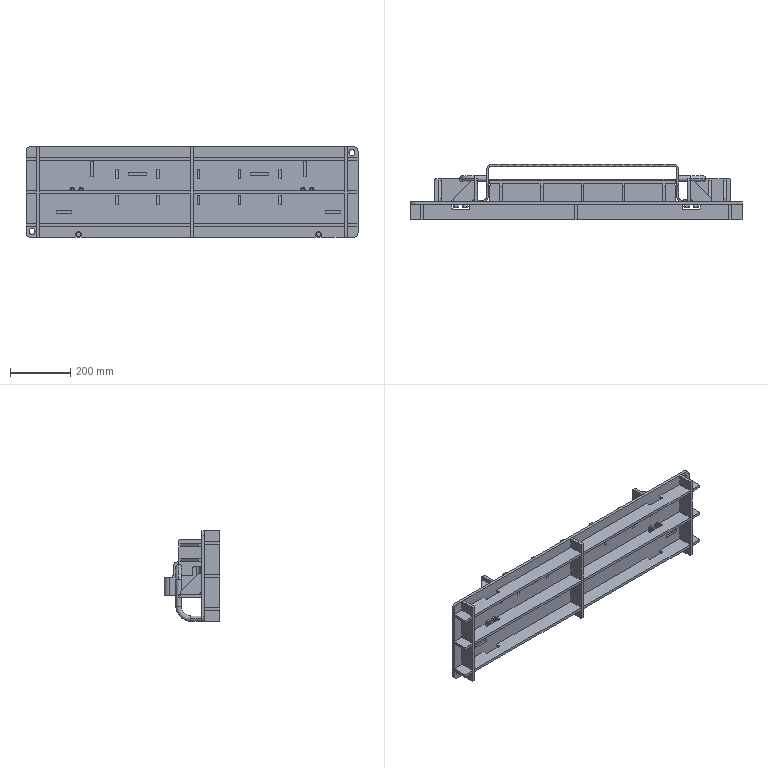Part | SolidWorks | features ReferencePattern 16, LocalLPattern 6, MirrorCompFeat 1 | 39 solids | 1349 faces | box 1100 x 184 x 300 mm | volume 7919569 mm3 | plane 883 | cylinder 262 | cone 196 | torus 8 | commonest cylinder face diameters 8.376 x56 4 x53 10 x34 15 x24 20 x21 6 x20